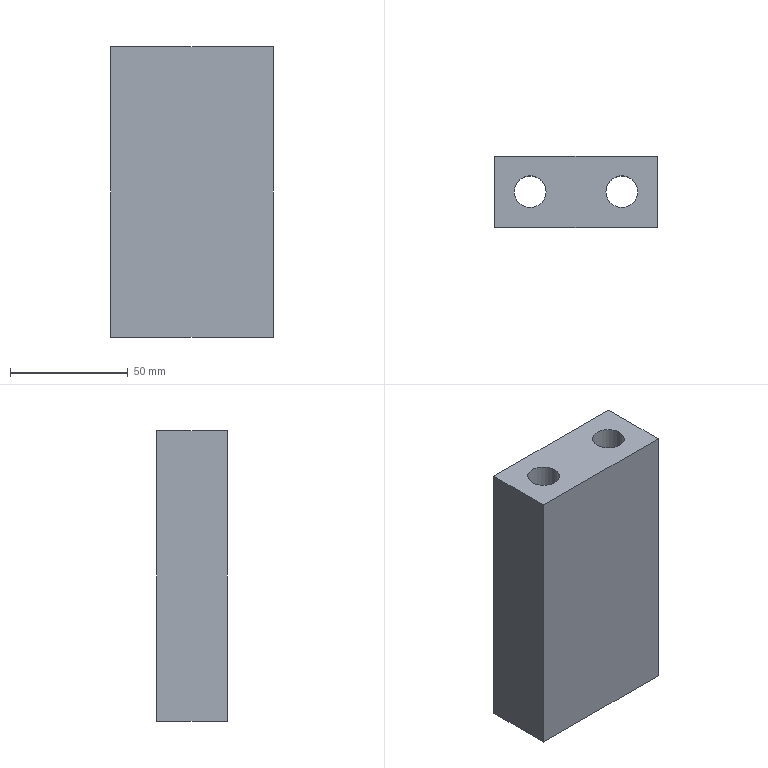Part | NX | features LIN_SOLID_COLOR 2 | 1 solid | 12 faces | box 69 x 30 x 123.5 mm | volume 188309 mm3 | plane 8 | cylinder 4 | commonest cylinder face diameters 13.5 x2 20 x2
STEP:
#1=CARTESIAN_POINT('',(671.,0.,-136.5));
#2=VERTEX_POINT('',#1);
#3=CARTESIAN_POINT('',(661.,0.,-136.5));
#4=DIRECTION('',(0.,0.,1.));
#5=DIRECTION('',(1.,0.,0.));
#6=AXIS2_PLACEMENT_3D('',#3,#4,#5);
#7=CIRCLE('',#6,10.);
#8=EDGE_CURVE('',#2,#2,#7,.T.);
#9=ORIENTED_EDGE('',*,*,#8,.F.);
#10=EDGE_LOOP('',(#9));
#11=FACE_BOUND('',#10,.T.);
#12=CARTESIAN_POINT('',(667.75,0.,-136.5));
#13=VERTEX_POINT('',#12);
#14=CARTESIAN_POINT('',(661.,0.,-136.5));
#15=DIRECTION('',(0.,0.,1.));
#16=DIRECTION('',(1.,0.,0.));
#17=AXIS2_PLACEMENT_3D('',#14,#15,#16);
#18=CIRCLE('',#17,6.75);
#19=EDGE_CURVE('',#13,#13,#18,.T.);
#20=ORIENTED_EDGE('',*,*,#19,.T.);
#21=EDGE_LOOP('',(#20));
#22=FACE_BOUND('',#21,.T.);
#23=CARTESIAN_POINT('',(622.,0.,-136.5));
#24=DIRECTION('',(0.,0.,1.));
#25=DIRECTION('',(1.,0.,0.));
#26=AXIS2_PLACEMENT_3D('',#23,#24,#25);
#27=PLANE('',#26);
#28=ADVANCED_FACE('',(#11,#22),#27,.F.);
#29=CARTESIAN_POINT('',(632.,0.,-136.5));
#30=VERTEX_POINT('',#29);
#31=CARTESIAN_POINT('',(622.,0.,-136.5));
#32=DIRECTION('',(0.,0.,-1.));
#33=DIRECTION('',(1.,0.,0.));
#34=AXIS2_PLACEMENT_3D('',#31,#32,#33);
#35=CIRCLE('',#34,10.);
#36=EDGE_CURVE('',#30,#30,#35,.F.);
#37=ORIENTED_EDGE('',*,*,#36,.F.);
#38=EDGE_LOOP('',(#37));
#39=FACE_BOUND('',#38,.T.);
#40=CARTESIAN_POINT('',(628.75,0.,-136.5));
#41=VERTEX_POINT('',#40);
#42=CARTESIAN_POINT('',(622.,0.,-136.5));
#43=DIRECTION('',(0.,0.,1.));
#44=DIRECTION('',(1.,0.,0.));
#45=AXIS2_PLACEMENT_3D('',#42,#43,#44);
#46=CIRCLE('',#45,6.75);
#47=EDGE_CURVE('',#41,#41,#46,.T.);
#48=ORIENTED_EDGE('',*,*,#47,.T.);
#49=EDGE_LOOP('',(#48));
#50=FACE_BOUND('',#49,.T.);
#51=CARTESIAN_POINT('',(622.,0.,-136.5));
#52=DIRECTION('',(0.,0.,1.));
#53=DIRECTION('',(1.,0.,0.));
#54=AXIS2_PLACEMENT_3D('',#51,#52,#53);
#55=PLANE('',#54);
#56=ADVANCED_FACE('',(#39,#50),#55,.F.);
#57=CARTESIAN_POINT('',(607.,-15.,-106.5));
#58=VERTEX_POINT('',#57);
#59=CARTESIAN_POINT('',(607.,15.,-106.5));
#60=VERTEX_POINT('',#59);
#61=CARTESIAN_POINT('',(607.,20.,-106.5));
#62=DIRECTION('',(0.,1.,0.));
#63=VECTOR('',#62,1000.);
#64=LINE('',#61,#63);
#65=EDGE_CURVE('',#58,#60,#64,.T.);
#66=ORIENTED_EDGE('',*,*,#65,.T.);
#67=CARTESIAN_POINT('',(607.,15.,-230.));
#68=VERTEX_POINT('',#67);
#69=CARTESIAN_POINT('',(607.,15.,-101.5));
#70=DIRECTION('',(0.,0.,1.));
#71=VECTOR('',#70,1000.);
#72=LINE('',#69,#71);
#73=EDGE_CURVE('',#68,#60,#72,.T.);
#74=ORIENTED_EDGE('',*,*,#73,.F.);
#75=CARTESIAN_POINT('',(607.,-15.,-230.));
#76=VERTEX_POINT('',#75);
#77=CARTESIAN_POINT('',(607.,0.,-230.));
#78=DIRECTION('',(0.,1.,0.));
#79=VECTOR('',#78,1000.);
#80=LINE('',#77,#79);
#81=EDGE_CURVE('',#76,#68,#80,.T.);
#82=ORIENTED_EDGE('',*,*,#81,.F.);
#83=CARTESIAN_POINT('',(607.,-15.,-101.5));
#84=DIRECTION('',(0.,0.,1.));
#85=VECTOR('',#84,1000.);
#86=LINE('',#83,#85);
#87=EDGE_CURVE('',#76,#58,#86,.T.);
#88=ORIENTED_EDGE('',*,*,#87,.T.);
#89=EDGE_LOOP('',(#66,#74,#82,#88));
#90=FACE_BOUND('',#89,.T.);
#91=CARTESIAN_POINT('',(607.,20.,-101.5));
#92=DIRECTION('',(1.,0.,0.));
#93=DIRECTION('',(0.,0.,1.));
#94=AXIS2_PLACEMENT_3D('',#91,#92,#93);
#95=PLANE('',#94);
#96=ADVANCED_FACE('',(#90),#95,.F.);
#97=CARTESIAN_POINT('',(676.,15.,-106.5));
#98=VERTEX_POINT('',#97);
#99=CARTESIAN_POINT('',(446.,15.,-106.5));
#100=DIRECTION('',(-1.,0.,0.));
#101=VECTOR('',#100,1000.);
#102=LINE('',#99,#101);
#103=EDGE_CURVE('',#98,#60,#102,.T.);
#104=ORIENTED_EDGE('',*,*,#103,.F.);
#105=CARTESIAN_POINT('',(676.,15.,-230.));
#106=VERTEX_POINT('',#105);
#107=CARTESIAN_POINT('',(676.,15.,-101.5));
#108=DIRECTION('',(0.,0.,-1.));
#109=VECTOR('',#108,1000.);
#110=LINE('',#107,#109);
#111=EDGE_CURVE('',#106,#98,#110,.F.);
#112=ORIENTED_EDGE('',*,*,#111,.F.);
#113=CARTESIAN_POINT('',(426.,15.,-230.));
#114=DIRECTION('',(1.,0.,0.));
#115=VECTOR('',#114,1000.);
#116=LINE('',#113,#115);
#117=EDGE_CURVE('',#68,#106,#116,.T.);
#118=ORIENTED_EDGE('',*,*,#117,.F.);
#119=ORIENTED_EDGE('',*,*,#73,.T.);
#120=EDGE_LOOP('',(#104,#112,#118,#119));
#121=FACE_BOUND('',#120,.T.);
#122=CARTESIAN_POINT('',(446.,15.,-101.5));
#123=DIRECTION('',(0.,-1.,0.));
#124=DIRECTION('',(0.,0.,1.));
#125=AXIS2_PLACEMENT_3D('',#122,#123,#124);
#126=PLANE('',#125);
#127=ADVANCED_FACE('',(#121),#126,.F.);
#128=CARTESIAN_POINT('',(676.,-15.,-230.));
#129=VERTEX_POINT('',#128);
#130=CARTESIAN_POINT('',(676.,-15.,-106.5));
#131=VERTEX_POINT('',#130);
#132=CARTESIAN_POINT('',(676.,-15.,-101.5));
#133=DIRECTION('',(0.,0.,-1.));
#134=VECTOR('',#133,1000.);
#135=LINE('',#132,#134);
#136=EDGE_CURVE('',#129,#131,#135,.F.);
#137=ORIENTED_EDGE('',*,*,#136,.T.);
#138=CARTESIAN_POINT('',(446.,-15.,-106.5));
#139=DIRECTION('',(-1.,0.,0.));
#140=VECTOR('',#139,1000.);
#141=LINE('',#138,#140);
#142=EDGE_CURVE('',#131,#58,#141,.T.);
#143=ORIENTED_EDGE('',*,*,#142,.T.);
#144=ORIENTED_EDGE('',*,*,#87,.F.);
#145=CARTESIAN_POINT('',(426.,-15.,-230.));
#146=DIRECTION('',(1.,0.,0.));
#147=VECTOR('',#146,1000.);
#148=LINE('',#145,#147);
#149=EDGE_CURVE('',#76,#129,#148,.T.);
#150=ORIENTED_EDGE('',*,*,#149,.T.);
#151=EDGE_LOOP('',(#137,#143,#144,#150));
#152=FACE_BOUND('',#151,.T.);
#153=CARTESIAN_POINT('',(446.,-15.,-101.5));
#154=DIRECTION('',(0.,-1.,0.));
#155=DIRECTION('',(0.,0.,1.));
#156=AXIS2_PLACEMENT_3D('',#153,#154,#155);
#157=PLANE('',#156);
#158=ADVANCED_FACE('',(#152),#157,.T.);
#159=CARTESIAN_POINT('',(671.,0.,-230.));
#160=VERTEX_POINT('',#159);
#161=CARTESIAN_POINT('',(661.,0.,-230.));
#162=DIRECTION('',(0.,0.,1.));
#163=DIRECTION('',(1.,0.,0.));
#164=AXIS2_PLACEMENT_3D('',#161,#162,#163);
#165=CIRCLE('',#164,10.);
#166=EDGE_CURVE('',#160,#160,#165,.T.);
#167=ORIENTED_EDGE('',*,*,#166,.T.);
#168=EDGE_LOOP('',(#167));
#169=FACE_BOUND('',#168,.T.);
#170=CARTESIAN_POINT('',(632.,0.,-230.));
#171=VERTEX_POINT('',#170);
#172=CARTESIAN_POINT('',(622.,0.,-230.));
#173=DIRECTION('',(0.,0.,1.));
#174=DIRECTION('',(1.,0.,0.));
#175=AXIS2_PLACEMENT_3D('',#172,#173,#174);
#176=CIRCLE('',#175,10.);
#177=EDGE_CURVE('',#171,#171,#176,.T.);
#178=ORIENTED_EDGE('',*,*,#177,.T.);
#179=EDGE_LOOP('',(#178));
#180=FACE_BOUND('',#179,.T.);
#181=ORIENTED_EDGE('',*,*,#117,.T.);
#182=CARTESIAN_POINT('',(676.,20.,-230.));
#183=DIRECTION('',(0.,-1.,0.));
#184=VECTOR('',#183,1000.);
#185=LINE('',#182,#184);
#186=EDGE_CURVE('',#129,#106,#185,.F.);
#187=ORIENTED_EDGE('',*,*,#186,.F.);
#188=ORIENTED_EDGE('',*,*,#149,.F.);
#189=ORIENTED_EDGE('',*,*,#81,.T.);
#190=EDGE_LOOP('',(#181,#187,#188,#189));
#191=FACE_BOUND('',#190,.T.);
#192=CARTESIAN_POINT('',(426.,0.,-230.));
#193=DIRECTION('',(0.,0.,1.));
#194=DIRECTION('',(-1.,0.,0.));
#195=AXIS2_PLACEMENT_3D('',#192,#193,#194);
#196=PLANE('',#195);
#197=ADVANCED_FACE('',(#169,#180,#191),#196,.F.);
#198=CARTESIAN_POINT('',(667.75,0.,-106.5));
#199=VERTEX_POINT('',#198);
#200=CARTESIAN_POINT('',(661.,0.,-106.5));
#201=DIRECTION('',(0.,0.,-1.));
#202=DIRECTION('',(1.,0.,0.));
#203=AXIS2_PLACEMENT_3D('',#200,#201,#202);
#204=CIRCLE('',#203,6.75);
#205=EDGE_CURVE('',#199,#199,#204,.T.);
#206=ORIENTED_EDGE('',*,*,#205,.T.);
#207=EDGE_LOOP('',(#206));
#208=FACE_BOUND('',#207,.T.);
#209=CARTESIAN_POINT('',(628.75,0.,-106.5));
#210=VERTEX_POINT('',#209);
#211=CARTESIAN_POINT('',(622.,0.,-106.5));
#212=DIRECTION('',(0.,0.,-1.));
#213=DIRECTION('',(1.,0.,0.));
#214=AXIS2_PLACEMENT_3D('',#211,#212,#213);
#215=CIRCLE('',#214,6.75);
#216=EDGE_CURVE('',#210,#210,#215,.T.);
#217=ORIENTED_EDGE('',*,*,#216,.T.);
#218=EDGE_LOOP('',(#217));
#219=FACE_BOUND('',#218,.T.);
#220=CARTESIAN_POINT('',(676.,750.,-106.5));
#221=DIRECTION('',(0.,-1.,0.));
#222=VECTOR('',#221,1000.);
#223=LINE('',#220,#222);
#224=EDGE_CURVE('',#131,#98,#223,.F.);
#225=ORIENTED_EDGE('',*,*,#224,.T.);
#226=ORIENTED_EDGE('',*,*,#103,.T.);
#227=ORIENTED_EDGE('',*,*,#65,.F.);
#228=ORIENTED_EDGE('',*,*,#142,.F.);
#229=EDGE_LOOP('',(#225,#226,#227,#228));
#230=FACE_BOUND('',#229,.T.);
#231=CARTESIAN_POINT('',(446.,750.,-106.5));
#232=DIRECTION('',(0.,0.,-1.));
#233=DIRECTION('',(0.,-1.,0.));
#234=AXIS2_PLACEMENT_3D('',#231,#232,#233);
#235=PLANE('',#234);
#236=ADVANCED_FACE('',(#208,#219,#230),#235,.F.);
#237=ORIENTED_EDGE('',*,*,#186,.T.);
#238=ORIENTED_EDGE('',*,*,#111,.T.);
#239=ORIENTED_EDGE('',*,*,#224,.F.);
#240=ORIENTED_EDGE('',*,*,#136,.F.);
#241=EDGE_LOOP('',(#237,#238,#239,#240));
#242=FACE_BOUND('',#241,.T.);
#243=CARTESIAN_POINT('',(676.,20.,-101.5));
#244=DIRECTION('',(1.,0.,0.));
#245=DIRECTION('',(0.,0.,1.));
#246=AXIS2_PLACEMENT_3D('',#243,#244,#245);
#247=PLANE('',#246);
#248=ADVANCED_FACE('',(#242),#247,.T.);
#249=ORIENTED_EDGE('',*,*,#36,.T.);
#250=EDGE_LOOP('',(#249));
#251=FACE_BOUND('',#250,.T.);
#252=ORIENTED_EDGE('',*,*,#177,.F.);
#253=EDGE_LOOP('',(#252));
#254=FACE_BOUND('',#253,.T.);
#255=CARTESIAN_POINT('',(622.,0.,-190.));
#256=DIRECTION('',(0.,0.,1.));
#257=DIRECTION('',(1.,0.,0.));
#258=AXIS2_PLACEMENT_3D('',#255,#256,#257);
#259=CYLINDRICAL_SURFACE('',#258,10.);
#260=ADVANCED_FACE('',(#251,#254),#259,.F.);
#261=ORIENTED_EDGE('',*,*,#216,.F.);
#262=EDGE_LOOP('',(#261));
#263=FACE_BOUND('',#262,.T.);
#264=ORIENTED_EDGE('',*,*,#47,.F.);
#265=EDGE_LOOP('',(#264));
#266=FACE_BOUND('',#265,.T.);
#267=CARTESIAN_POINT('',(622.,0.,-190.));
#268=DIRECTION('',(0.,0.,1.));
#269=DIRECTION('',(1.,0.,0.));
#270=AXIS2_PLACEMENT_3D('',#267,#268,#269);
#271=CYLINDRICAL_SURFACE('',#270,6.75);
#272=ADVANCED_FACE('',(#263,#266),#271,.F.);
#273=ORIENTED_EDGE('',*,*,#8,.T.);
#274=EDGE_LOOP('',(#273));
#275=FACE_BOUND('',#274,.T.);
#276=ORIENTED_EDGE('',*,*,#166,.F.);
#277=EDGE_LOOP('',(#276));
#278=FACE_BOUND('',#277,.T.);
#279=CARTESIAN_POINT('',(661.,0.,-190.));
#280=DIRECTION('',(0.,0.,1.));
#281=DIRECTION('',(1.,0.,0.));
#282=AXIS2_PLACEMENT_3D('',#279,#280,#281);
#283=CYLINDRICAL_SURFACE('',#282,10.);
#284=ADVANCED_FACE('',(#275,#278),#283,.F.);
#285=ORIENTED_EDGE('',*,*,#205,.F.);
#286=EDGE_LOOP('',(#285));
#287=FACE_BOUND('',#286,.T.);
#288=ORIENTED_EDGE('',*,*,#19,.F.);
#289=EDGE_LOOP('',(#288));
#290=FACE_BOUND('',#289,.T.);
#291=CARTESIAN_POINT('',(661.,0.,-190.));
#292=DIRECTION('',(0.,0.,1.));
#293=DIRECTION('',(1.,0.,0.));
#294=AXIS2_PLACEMENT_3D('',#291,#292,#293);
#295=CYLINDRICAL_SURFACE('',#294,6.75);
#296=ADVANCED_FACE('',(#287,#290),#295,.F.);
#297=CLOSED_SHELL('',(#28,#56,#96,#127,#158,#197,#236,#248,#260,#272,#284,#296));
#298=MANIFOLD_SOLID_BREP('',#297);
#299=(LENGTH_UNIT()NAMED_UNIT(*)SI_UNIT(.MILLI.,.METRE.));
#300=UNCERTAINTY_MEASURE_WITH_UNIT(LENGTH_MEASURE(0.00001),#299,'','');
#301=(NAMED_UNIT(*)PLANE_ANGLE_UNIT()SI_UNIT($,.RADIAN.));
#302=(NAMED_UNIT(*)SI_UNIT($,.STERADIAN.)SOLID_ANGLE_UNIT());
#303=(GEOMETRIC_REPRESENTATION_CONTEXT(3)GLOBAL_UNCERTAINTY_ASSIGNED_CONTEXT((#300))GLOBAL_UNIT_ASSIGNED_CONTEXT((#299,#301,#302))REPRESENTATION_CONTEXT('',''));
#304=ADVANCED_BREP_SHAPE_REPRESENTATION('',(#298),#303);